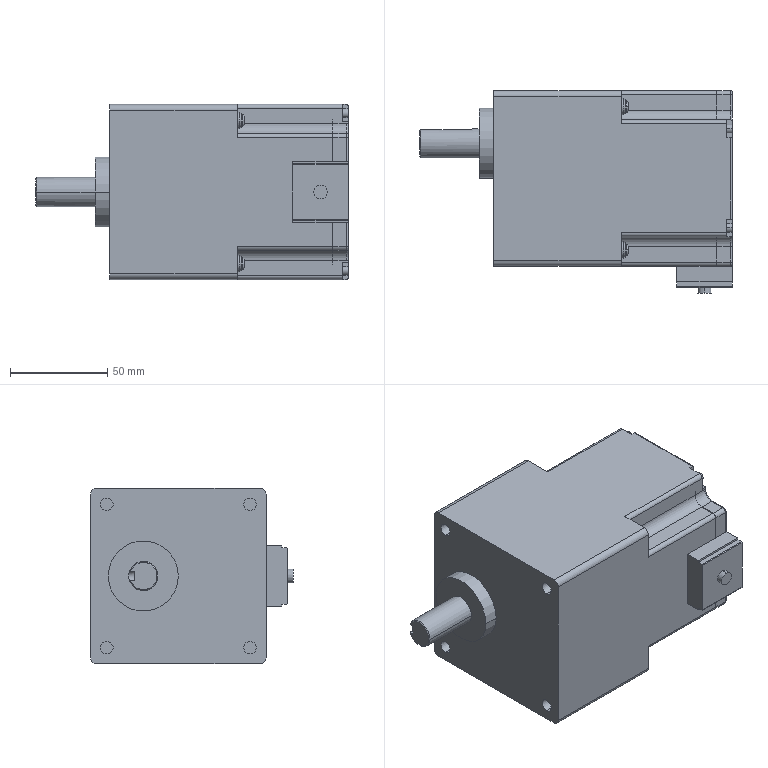Part | STEP file | 1.6米90W | 2 solids | 178 faces | box 160.5 x 104 x 90 mm | volume 953973 mm3 | cylinder 83 | plane 78 | spline 16 | cone 1 | commonest cylinder face diameters 2 x12 4 x12 6 x12 4.5 x8 6.5 x8 7.5 x8